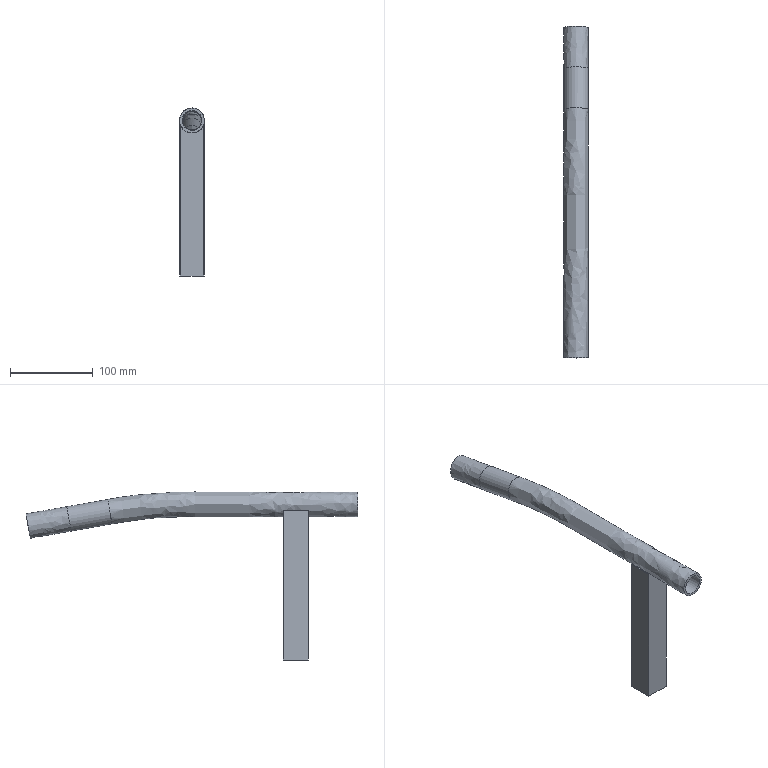Part | NX | features solid 2 | 1 solid | 22 faces | box 30 x 400.326 x 202.586 mm | volume 133159 mm3 | plane 15 | spline 4 | cylinder 3 | commonest cylinder face diameters 30 x2 24 x1
STEP:
#1=CARTESIAN_POINT('',(-482.491,1164.,-350.));
#2=VERTEX_POINT('',#1);
#3=CARTESIAN_POINT('',(-456.509,1164.,-350.));
#4=VERTEX_POINT('',#3);
#5=CARTESIAN_POINT('',(-482.491,1164.,-350.));
#6=CARTESIAN_POINT('',(-481.169,1164.,-352.288));
#7=CARTESIAN_POINT('',(-477.363,1164.,-356.084));
#8=CARTESIAN_POINT('',(-469.496,1164.,-358.205));
#9=CARTESIAN_POINT('',(-461.661,1164.,-356.096));
#10=CARTESIAN_POINT('',(-457.831,1164.,-352.288));
#11=CARTESIAN_POINT('',(-456.509,1164.,-350.));
#12=B_SPLINE_CURVE_WITH_KNOTS('',3,(#5,#6,#7,#8,#9,#10,#11),.UNSPECIFIED.,.F.,.F.,(4,1,1,1,4),(0.,0.007815,0.01563,0.02344,0.03126),.UNSPECIFIED.);
#13=EDGE_CURVE('',#2,#4,#12,.T.);
#14=ORIENTED_EDGE('',*,*,#13,.T.);
#15=CARTESIAN_POINT('',(-454.5,1164.,-350.));
#16=VERTEX_POINT('',#15);
#17=CARTESIAN_POINT('',(-454.5,1164.,-350.));
#18=DIRECTION('',(1.,0.,0.));
#19=VECTOR('',#18,1000.);
#20=LINE('',#17,#19);
#21=EDGE_CURVE('',#16,#4,#20,.F.);
#22=ORIENTED_EDGE('',*,*,#21,.F.);
#23=CARTESIAN_POINT('',(-454.5,1164.,-530.));
#24=VERTEX_POINT('',#23);
#25=CARTESIAN_POINT('',(-454.5,1164.,-635.));
#26=DIRECTION('',(0.,0.,1.));
#27=VECTOR('',#26,1000.);
#28=LINE('',#25,#27);
#29=EDGE_CURVE('',#24,#16,#28,.T.);
#30=ORIENTED_EDGE('',*,*,#29,.F.);
#31=CARTESIAN_POINT('',(-484.5,1164.,-530.));
#32=VERTEX_POINT('',#31);
#33=CARTESIAN_POINT('',(-451.75,1164.,-530.));
#34=DIRECTION('',(1.,0.,0.));
#35=VECTOR('',#34,1000.);
#36=LINE('',#33,#35);
#37=EDGE_CURVE('',#24,#32,#36,.F.);
#38=ORIENTED_EDGE('',*,*,#37,.T.);
#39=CARTESIAN_POINT('',(-484.5,1164.,-350.));
#40=VERTEX_POINT('',#39);
#41=CARTESIAN_POINT('',(-484.5,1164.,-635.));
#42=DIRECTION('',(0.,0.,-1.));
#43=VECTOR('',#42,1000.);
#44=LINE('',#41,#43);
#45=EDGE_CURVE('',#32,#40,#44,.F.);
#46=ORIENTED_EDGE('',*,*,#45,.T.);
#47=CARTESIAN_POINT('',(-454.5,1164.,-350.));
#48=DIRECTION('',(1.,0.,0.));
#49=VECTOR('',#48,1000.);
#50=LINE('',#47,#49);
#51=EDGE_CURVE('',#2,#40,#50,.F.);
#52=ORIENTED_EDGE('',*,*,#51,.F.);
#53=EDGE_LOOP('',(#14,#22,#30,#38,#46,#52));
#54=FACE_BOUND('',#53,.T.);
#55=CARTESIAN_POINT('',(-451.75,1164.,-635.));
#56=DIRECTION('',(0.,-1.,0.));
#57=DIRECTION('',(-1.,0.,0.));
#58=AXIS2_PLACEMENT_3D('',#55,#56,#57);
#59=PLANE('',#58);
#60=ADVANCED_FACE('',(#54),#59,.F.);
#61=CARTESIAN_POINT('',(-456.51,1162.5,-350.));
#62=VERTEX_POINT('',#61);
#63=CARTESIAN_POINT('',(-482.49,1162.5,-350.));
#64=VERTEX_POINT('',#63);
#65=CARTESIAN_POINT('',(-456.51,1162.5,-350.));
#66=CARTESIAN_POINT('',(-457.831,1162.5,-352.288));
#67=CARTESIAN_POINT('',(-461.637,1162.5,-356.084));
#68=CARTESIAN_POINT('',(-469.504,1162.5,-358.205));
#69=CARTESIAN_POINT('',(-477.339,1162.5,-356.096));
#70=CARTESIAN_POINT('',(-481.169,1162.5,-352.288));
#71=CARTESIAN_POINT('',(-482.49,1162.5,-350.));
#72=B_SPLINE_CURVE_WITH_KNOTS('',3,(#65,#66,#67,#68,#69,#70,#71),.UNSPECIFIED.,.F.,.F.,(4,1,1,1,4),(0.,0.007814,0.01563,0.02344,0.03126),.UNSPECIFIED.);
#73=EDGE_CURVE('',#62,#64,#72,.T.);
#74=ORIENTED_EDGE('',*,*,#73,.T.);
#75=CARTESIAN_POINT('',(-483.,1162.5,-350.));
#76=VERTEX_POINT('',#75);
#77=CARTESIAN_POINT('',(-451.75,1162.5,-350.));
#78=DIRECTION('',(1.,0.,0.));
#79=VECTOR('',#78,1000.);
#80=LINE('',#77,#79);
#81=EDGE_CURVE('',#76,#64,#80,.T.);
#82=ORIENTED_EDGE('',*,*,#81,.F.);
#83=CARTESIAN_POINT('',(-483.,1162.5,-530.));
#84=VERTEX_POINT('',#83);
#85=CARTESIAN_POINT('',(-483.,1162.5,-285.));
#86=DIRECTION('',(0.,0.,-1.));
#87=VECTOR('',#86,1000.);
#88=LINE('',#85,#87);
#89=EDGE_CURVE('',#76,#84,#88,.T.);
#90=ORIENTED_EDGE('',*,*,#89,.T.);
#91=CARTESIAN_POINT('',(-456.,1162.5,-530.));
#92=VERTEX_POINT('',#91);
#93=CARTESIAN_POINT('',(-451.75,1162.5,-530.));
#94=DIRECTION('',(-1.,0.,0.));
#95=VECTOR('',#94,1000.);
#96=LINE('',#93,#95);
#97=EDGE_CURVE('',#84,#92,#96,.F.);
#98=ORIENTED_EDGE('',*,*,#97,.T.);
#99=CARTESIAN_POINT('',(-456.,1162.5,-350.));
#100=VERTEX_POINT('',#99);
#101=CARTESIAN_POINT('',(-456.,1162.5,-285.));
#102=DIRECTION('',(0.,0.,-1.));
#103=VECTOR('',#102,1000.);
#104=LINE('',#101,#103);
#105=EDGE_CURVE('',#100,#92,#104,.T.);
#106=ORIENTED_EDGE('',*,*,#105,.F.);
#107=CARTESIAN_POINT('',(-451.75,1162.5,-350.));
#108=DIRECTION('',(1.,0.,0.));
#109=VECTOR('',#108,1000.);
#110=LINE('',#107,#109);
#111=EDGE_CURVE('',#62,#100,#110,.T.);
#112=ORIENTED_EDGE('',*,*,#111,.F.);
#113=EDGE_LOOP('',(#74,#82,#90,#98,#106,#112));
#114=FACE_BOUND('',#113,.T.);
#115=CARTESIAN_POINT('',(-451.75,1162.5,-285.));
#116=DIRECTION('',(0.,1.,0.));
#117=DIRECTION('',(1.,0.,0.));
#118=AXIS2_PLACEMENT_3D('',#115,#116,#117);
#119=PLANE('',#118);
#120=ADVANCED_FACE('',(#114),#119,.F.);
#121=CARTESIAN_POINT('',(-482.491,1164.,-350.));
#122=CARTESIAN_POINT('',(-482.49,1163.5,-350.));
#123=CARTESIAN_POINT('',(-482.49,1163.,-350.));
#124=CARTESIAN_POINT('',(-482.49,1162.5,-350.));
#125=B_SPLINE_CURVE_WITH_KNOTS('',3,(#121,#122,#123,#124),.UNSPECIFIED.,.F.,.F.,(4,4),(0.,0.0015),.UNSPECIFIED.);
#126=EDGE_CURVE('',#64,#2,#125,.F.);
#127=ORIENTED_EDGE('',*,*,#126,.T.);
#128=ORIENTED_EDGE('',*,*,#51,.T.);
#129=CARTESIAN_POINT('',(-484.5,1134.,-350.));
#130=VERTEX_POINT('',#129);
#131=CARTESIAN_POINT('',(-484.5,1134.,-350.));
#132=DIRECTION('',(0.,1.,0.));
#133=VECTOR('',#132,1000.);
#134=LINE('',#131,#133);
#135=EDGE_CURVE('',#40,#130,#134,.F.);
#136=ORIENTED_EDGE('',*,*,#135,.T.);
#137=CARTESIAN_POINT('',(-482.49,1134.,-350.));
#138=VERTEX_POINT('',#137);
#139=CARTESIAN_POINT('',(-454.5,1134.,-350.));
#140=DIRECTION('',(1.,0.,0.));
#141=VECTOR('',#140,1000.);
#142=LINE('',#139,#141);
#143=EDGE_CURVE('',#138,#130,#142,.F.);
#144=ORIENTED_EDGE('',*,*,#143,.F.);
#145=CARTESIAN_POINT('',(-482.49,1135.5,-350.));
#146=VERTEX_POINT('',#145);
#147=CARTESIAN_POINT('',(-482.49,764.,-350.));
#148=DIRECTION('',(0.,1.,0.));
#149=VECTOR('',#148,1000.);
#150=LINE('',#147,#149);
#151=EDGE_CURVE('',#138,#146,#150,.T.);
#152=ORIENTED_EDGE('',*,*,#151,.T.);
#153=CARTESIAN_POINT('',(-483.,1135.5,-350.));
#154=VERTEX_POINT('',#153);
#155=CARTESIAN_POINT('',(-451.75,1135.5,-350.));
#156=DIRECTION('',(1.,0.,0.));
#157=VECTOR('',#156,1000.);
#158=LINE('',#155,#157);
#159=EDGE_CURVE('',#154,#146,#158,.T.);
#160=ORIENTED_EDGE('',*,*,#159,.F.);
#161=CARTESIAN_POINT('',(-483.,1134.,-350.));
#162=DIRECTION('',(0.,-1.,0.));
#163=VECTOR('',#162,1000.);
#164=LINE('',#161,#163);
#165=EDGE_CURVE('',#76,#154,#164,.T.);
#166=ORIENTED_EDGE('',*,*,#165,.F.);
#167=ORIENTED_EDGE('',*,*,#81,.T.);
#168=EDGE_LOOP('',(#127,#128,#136,#144,#152,#160,#166,#167));
#169=FACE_BOUND('',#168,.T.);
#170=CARTESIAN_POINT('',(-454.5,1134.,-350.));
#171=DIRECTION('',(0.,0.,-1.));
#172=DIRECTION('',(0.,-1.,0.));
#173=AXIS2_PLACEMENT_3D('',#170,#171,#172);
#174=PLANE('',#173);
#175=ADVANCED_FACE('',(#169),#174,.F.);
#176=CARTESIAN_POINT('',(-456.509,1164.,-350.));
#177=CARTESIAN_POINT('',(-456.51,1163.5,-350.));
#178=CARTESIAN_POINT('',(-456.51,1163.,-350.));
#179=CARTESIAN_POINT('',(-456.51,1162.5,-350.));
#180=B_SPLINE_CURVE_WITH_KNOTS('',3,(#176,#177,#178,#179),.UNSPECIFIED.,.F.,.F.,(4,4),(0.,0.0015),.UNSPECIFIED.);
#181=EDGE_CURVE('',#4,#62,#180,.T.);
#182=ORIENTED_EDGE('',*,*,#181,.T.);
#183=ORIENTED_EDGE('',*,*,#111,.T.);
#184=CARTESIAN_POINT('',(-456.,1135.5,-350.));
#185=VERTEX_POINT('',#184);
#186=CARTESIAN_POINT('',(-456.,1134.,-350.));
#187=DIRECTION('',(0.,-1.,0.));
#188=VECTOR('',#187,1000.);
#189=LINE('',#186,#188);
#190=EDGE_CURVE('',#100,#185,#189,.T.);
#191=ORIENTED_EDGE('',*,*,#190,.T.);
#192=CARTESIAN_POINT('',(-456.51,1135.5,-350.));
#193=VERTEX_POINT('',#192);
#194=CARTESIAN_POINT('',(-451.75,1135.5,-350.));
#195=DIRECTION('',(1.,0.,0.));
#196=VECTOR('',#195,1000.);
#197=LINE('',#194,#196);
#198=EDGE_CURVE('',#193,#185,#197,.T.);
#199=ORIENTED_EDGE('',*,*,#198,.F.);
#200=CARTESIAN_POINT('',(-456.51,1134.,-350.));
#201=VERTEX_POINT('',#200);
#202=CARTESIAN_POINT('',(-456.51,764.,-350.));
#203=DIRECTION('',(0.,1.,0.));
#204=VECTOR('',#203,1000.);
#205=LINE('',#202,#204);
#206=EDGE_CURVE('',#193,#201,#205,.F.);
#207=ORIENTED_EDGE('',*,*,#206,.T.);
#208=CARTESIAN_POINT('',(-454.5,1134.,-350.));
#209=VERTEX_POINT('',#208);
#210=CARTESIAN_POINT('',(-454.5,1134.,-350.));
#211=DIRECTION('',(1.,0.,0.));
#212=VECTOR('',#211,1000.);
#213=LINE('',#210,#212);
#214=EDGE_CURVE('',#209,#201,#213,.F.);
#215=ORIENTED_EDGE('',*,*,#214,.F.);
#216=CARTESIAN_POINT('',(-454.5,1134.,-350.));
#217=DIRECTION('',(0.,-1.,0.));
#218=VECTOR('',#217,1000.);
#219=LINE('',#216,#218);
#220=EDGE_CURVE('',#209,#16,#219,.F.);
#221=ORIENTED_EDGE('',*,*,#220,.T.);
#222=ORIENTED_EDGE('',*,*,#21,.T.);
#223=EDGE_LOOP('',(#182,#183,#191,#199,#207,#215,#221,#222));
#224=FACE_BOUND('',#223,.T.);
#225=CARTESIAN_POINT('',(-454.5,1134.,-350.));
#226=DIRECTION('',(0.,0.,-1.));
#227=DIRECTION('',(0.,-1.,0.));
#228=AXIS2_PLACEMENT_3D('',#225,#226,#227);
#229=PLANE('',#228);
#230=ADVANCED_FACE('',(#224),#229,.F.);
#231=CARTESIAN_POINT('',(-454.5,1134.,-530.));
#232=VERTEX_POINT('',#231);
#233=CARTESIAN_POINT('',(-454.5,1134.,-530.));
#234=DIRECTION('',(0.,-1.,0.));
#235=VECTOR('',#234,1000.);
#236=LINE('',#233,#235);
#237=EDGE_CURVE('',#232,#24,#236,.F.);
#238=ORIENTED_EDGE('',*,*,#237,.F.);
#239=CARTESIAN_POINT('',(-484.5,1134.,-530.));
#240=VERTEX_POINT('',#239);
#241=CARTESIAN_POINT('',(-451.75,1134.,-530.));
#242=DIRECTION('',(1.,0.,0.));
#243=VECTOR('',#242,1000.);
#244=LINE('',#241,#243);
#245=EDGE_CURVE('',#232,#240,#244,.F.);
#246=ORIENTED_EDGE('',*,*,#245,.T.);
#247=CARTESIAN_POINT('',(-484.5,1134.,-530.));
#248=DIRECTION('',(0.,1.,0.));
#249=VECTOR('',#248,1000.);
#250=LINE('',#247,#249);
#251=EDGE_CURVE('',#240,#32,#250,.T.);
#252=ORIENTED_EDGE('',*,*,#251,.T.);
#253=ORIENTED_EDGE('',*,*,#37,.F.);
#254=EDGE_LOOP('',(#238,#246,#252,#253));
#255=FACE_BOUND('',#254,.T.);
#256=CARTESIAN_POINT('',(-483.,1135.5,-530.));
#257=VERTEX_POINT('',#256);
#258=CARTESIAN_POINT('',(-483.,1134.,-530.));
#259=DIRECTION('',(0.,1.,0.));
#260=VECTOR('',#259,1000.);
#261=LINE('',#258,#260);
#262=EDGE_CURVE('',#84,#257,#261,.F.);
#263=ORIENTED_EDGE('',*,*,#262,.T.);
#264=CARTESIAN_POINT('',(-456.,1135.5,-530.));
#265=VERTEX_POINT('',#264);
#266=CARTESIAN_POINT('',(-451.75,1135.5,-530.));
#267=DIRECTION('',(-1.,0.,0.));
#268=VECTOR('',#267,1000.);
#269=LINE('',#266,#268);
#270=EDGE_CURVE('',#257,#265,#269,.F.);
#271=ORIENTED_EDGE('',*,*,#270,.T.);
#272=CARTESIAN_POINT('',(-456.,1134.,-530.));
#273=DIRECTION('',(0.,1.,0.));
#274=VECTOR('',#273,1000.);
#275=LINE('',#272,#274);
#276=EDGE_CURVE('',#92,#265,#275,.F.);
#277=ORIENTED_EDGE('',*,*,#276,.F.);
#278=ORIENTED_EDGE('',*,*,#97,.F.);
#279=EDGE_LOOP('',(#263,#271,#277,#278));
#280=FACE_BOUND('',#279,.T.);
#281=CARTESIAN_POINT('',(-451.75,1134.,-530.));
#282=DIRECTION('',(0.,0.,-1.));
#283=DIRECTION('',(-1.,0.,0.));
#284=AXIS2_PLACEMENT_3D('',#281,#282,#283);
#285=PLANE('',#284);
#286=ADVANCED_FACE('',(#255,#280),#285,.T.);
#287=ORIENTED_EDGE('',*,*,#45,.F.);
#288=ORIENTED_EDGE('',*,*,#251,.F.);
#289=CARTESIAN_POINT('',(-484.5,1134.,-635.));
#290=DIRECTION('',(0.,0.,-1.));
#291=VECTOR('',#290,1000.);
#292=LINE('',#289,#291);
#293=EDGE_CURVE('',#240,#130,#292,.F.);
#294=ORIENTED_EDGE('',*,*,#293,.T.);
#295=ORIENTED_EDGE('',*,*,#135,.F.);
#296=EDGE_LOOP('',(#287,#288,#294,#295));
#297=FACE_BOUND('',#296,.T.);
#298=CARTESIAN_POINT('',(-484.5,1134.,-635.));
#299=DIRECTION('',(-1.,0.,0.));
#300=DIRECTION('',(0.,0.,1.));
#301=AXIS2_PLACEMENT_3D('',#298,#299,#300);
#302=PLANE('',#301);
#303=ADVANCED_FACE('',(#297),#302,.T.);
#304=CARTESIAN_POINT('',(-454.5,1134.,-635.));
#305=DIRECTION('',(0.,0.,1.));
#306=VECTOR('',#305,1000.);
#307=LINE('',#304,#306);
#308=EDGE_CURVE('',#232,#209,#307,.T.);
#309=ORIENTED_EDGE('',*,*,#308,.F.);
#310=ORIENTED_EDGE('',*,*,#237,.T.);
#311=ORIENTED_EDGE('',*,*,#29,.T.);
#312=ORIENTED_EDGE('',*,*,#220,.F.);
#313=EDGE_LOOP('',(#309,#310,#311,#312));
#314=FACE_BOUND('',#313,.T.);
#315=CARTESIAN_POINT('',(-454.5,1134.,-635.));
#316=DIRECTION('',(-1.,0.,0.));
#317=DIRECTION('',(0.,0.,1.));
#318=AXIS2_PLACEMENT_3D('',#315,#316,#317);
#319=PLANE('',#318);
#320=ADVANCED_FACE('',(#314),#319,.F.);
#321=ORIENTED_EDGE('',*,*,#214,.T.);
#322=CARTESIAN_POINT('',(-469.5,1134.,-342.5));
#323=DIRECTION('',(0.,1.,0.));
#324=DIRECTION('',(-1.,0.,0.));
#325=AXIS2_PLACEMENT_3D('',#322,#323,#324);
#326=CIRCLE('',#325,15.);
#327=EDGE_CURVE('',#201,#138,#326,.T.);
#328=ORIENTED_EDGE('',*,*,#327,.T.);
#329=ORIENTED_EDGE('',*,*,#143,.T.);
#330=ORIENTED_EDGE('',*,*,#293,.F.);
#331=ORIENTED_EDGE('',*,*,#245,.F.);
#332=ORIENTED_EDGE('',*,*,#308,.T.);
#333=EDGE_LOOP('',(#321,#328,#329,#330,#331,#332));
#334=FACE_BOUND('',#333,.T.);
#335=CARTESIAN_POINT('',(-451.75,1134.,-635.));
#336=DIRECTION('',(0.,-1.,0.));
#337=DIRECTION('',(-1.,0.,0.));
#338=AXIS2_PLACEMENT_3D('',#335,#336,#337);
#339=PLANE('',#338);
#340=ADVANCED_FACE('',(#334),#339,.T.);
#341=ORIENTED_EDGE('',*,*,#165,.T.);
#342=CARTESIAN_POINT('',(-483.,1135.5,-285.));
#343=DIRECTION('',(0.,0.,-1.));
#344=VECTOR('',#343,1000.);
#345=LINE('',#342,#344);
#346=EDGE_CURVE('',#154,#257,#345,.T.);
#347=ORIENTED_EDGE('',*,*,#346,.T.);
#348=ORIENTED_EDGE('',*,*,#262,.F.);
#349=ORIENTED_EDGE('',*,*,#89,.F.);
#350=EDGE_LOOP('',(#341,#347,#348,#349));
#351=FACE_BOUND('',#350,.T.);
#352=CARTESIAN_POINT('',(-483.,1134.,-285.));
#353=DIRECTION('',(1.,0.,0.));
#354=DIRECTION('',(0.,-1.,0.));
#355=AXIS2_PLACEMENT_3D('',#352,#353,#354);
#356=PLANE('',#355);
#357=ADVANCED_FACE('',(#351),#356,.T.);
#358=ORIENTED_EDGE('',*,*,#105,.T.);
#359=ORIENTED_EDGE('',*,*,#276,.T.);
#360=CARTESIAN_POINT('',(-456.,1135.5,-285.));
#361=DIRECTION('',(0.,0.,-1.));
#362=VECTOR('',#361,1000.);
#363=LINE('',#360,#362);
#364=EDGE_CURVE('',#185,#265,#363,.T.);
#365=ORIENTED_EDGE('',*,*,#364,.F.);
#366=ORIENTED_EDGE('',*,*,#190,.F.);
#367=EDGE_LOOP('',(#358,#359,#365,#366));
#368=FACE_BOUND('',#367,.T.);
#369=CARTESIAN_POINT('',(-456.,1134.,-285.));
#370=DIRECTION('',(1.,0.,0.));
#371=DIRECTION('',(0.,-1.,0.));
#372=AXIS2_PLACEMENT_3D('',#369,#370,#371);
#373=PLANE('',#372);
#374=ADVANCED_FACE('',(#368),#373,.F.);
#375=ORIENTED_EDGE('',*,*,#159,.T.);
#376=CARTESIAN_POINT('',(-469.5,1135.5,-342.5));
#377=DIRECTION('',(0.,-1.,0.));
#378=DIRECTION('',(1.,0.,0.));
#379=AXIS2_PLACEMENT_3D('',#376,#377,#378);
#380=CIRCLE('',#379,15.);
#381=EDGE_CURVE('',#146,#193,#380,.T.);
#382=ORIENTED_EDGE('',*,*,#381,.T.);
#383=ORIENTED_EDGE('',*,*,#198,.T.);
#384=ORIENTED_EDGE('',*,*,#364,.T.);
#385=ORIENTED_EDGE('',*,*,#270,.F.);
#386=ORIENTED_EDGE('',*,*,#346,.F.);
#387=EDGE_LOOP('',(#375,#382,#383,#384,#385,#386));
#388=FACE_BOUND('',#387,.T.);
#389=CARTESIAN_POINT('',(-451.75,1135.5,-285.));
#390=DIRECTION('',(0.,1.,0.));
#391=DIRECTION('',(1.,0.,0.));
#392=AXIS2_PLACEMENT_3D('',#389,#390,#391);
#393=PLANE('',#392);
#394=ADVANCED_FACE('',(#388),#393,.T.);
#395=ORIENTED_EDGE('',*,*,#381,.F.);
#396=ORIENTED_EDGE('',*,*,#151,.F.);
#397=ORIENTED_EDGE('',*,*,#327,.F.);
#398=ORIENTED_EDGE('',*,*,#206,.F.);
#399=EDGE_LOOP('',(#395,#396,#397,#398));
#400=FACE_BOUND('',#399,.T.);
#401=CARTESIAN_POINT('',(-469.5,764.,-342.5));
#402=DIRECTION('',(0.,1.,0.));
#403=DIRECTION('',(1.,0.,0.));
#404=AXIS2_PLACEMENT_3D('',#401,#402,#403);
#405=CYLINDRICAL_SURFACE('',#404,15.);
#406=ADVANCED_FACE('',(#400),#405,.F.);
#407=CARTESIAN_POINT('',(-484.417,1074.,-344.075));
#408=VERTEX_POINT('',#407);
#409=CARTESIAN_POINT('',(-483.008,1074.,-349.869));
#410=CARTESIAN_POINT('',(-485.422,1074.,-342.193));
#411=CARTESIAN_POINT('',(-482.422,1074.,-332.049));
#412=CARTESIAN_POINT('',(-471.256,1074.,-325.971));
#413=CARTESIAN_POINT('',(-459.051,1074.,-329.569));
#414=CARTESIAN_POINT('',(-452.971,1074.,-340.753));
#415=CARTESIAN_POINT('',(-456.566,1074.,-352.937));
#416=CARTESIAN_POINT('',(-467.74,1074.,-359.035));
#417=CARTESIAN_POINT('',(-477.899,1074.,-356.018));
#418=CARTESIAN_POINT('',(-483.008,1074.,-349.869));
#419=CARTESIAN_POINT('',(-485.422,1074.,-342.193));
#420=CARTESIAN_POINT('',(-482.422,1074.,-332.049));
#421=B_SPLINE_CURVE_WITH_KNOTS('',3,(#409,#410,#411,#412,#413,#414,#415,#416,#417,#418,#419,#420),.UNSPECIFIED.,.T.,.F.,(1,1,1,1,1,1,1,1,1,1,1,1,1,1,1,1),(-0.02345,-0.01172,-0.005861,0.,0.01172,0.02345,0.03517,0.04689,0.05861,0.07034,0.08206,0.08792,0.09378,0.1055,0.1172,0.129),.UNSPECIFIED.);
#422=EDGE_CURVE('',#408,#408,#421,.T.);
#423=ORIENTED_EDGE('',*,*,#422,.T.);
#424=EDGE_LOOP('',(#423));
#425=FACE_BOUND('',#424,.T.);
#426=CARTESIAN_POINT('',(-454.5,1373.241,-351.177));
#427=VERTEX_POINT('',#426);
#428=CARTESIAN_POINT('',(-484.5,1373.241,-351.177));
#429=VERTEX_POINT('',#428);
#430=CARTESIAN_POINT('',(-454.5,1373.241,-351.177));
#431=CARTESIAN_POINT('',(-454.501,1372.897,-353.128));
#432=CARTESIAN_POINT('',(-455.286,1372.22,-356.97));
#433=CARTESIAN_POINT('',(-459.727,1371.06,-363.546));
#434=CARTESIAN_POINT('',(-469.485,1370.356,-367.54));
#435=CARTESIAN_POINT('',(-481.251,1371.2,-362.754));
#436=CARTESIAN_POINT('',(-484.499,1372.562,-355.032));
#437=CARTESIAN_POINT('',(-484.5,1373.241,-351.177));
#438=B_SPLINE_CURVE_WITH_KNOTS('',3,(#430,#431,#432,#433,#434,#435,#436,#437),.UNSPECIFIED.,.F.,.F.,(4,1,1,1,1,4),(0.000005601,0.005866,0.01173,0.02345,0.03517,0.04689),.UNSPECIFIED.);
#439=EDGE_CURVE('',#427,#429,#438,.T.);
#440=ORIENTED_EDGE('',*,*,#439,.F.);
#441=CARTESIAN_POINT('',(-484.5,1373.241,-351.177));
#442=CARTESIAN_POINT('',(-484.501,1373.921,-347.32));
#443=CARTESIAN_POINT('',(-481.266,1375.281,-339.61));
#444=CARTESIAN_POINT('',(-469.515,1376.13,-334.795));
#445=CARTESIAN_POINT('',(-457.752,1375.282,-339.605));
#446=CARTESIAN_POINT('',(-454.498,1373.93,-347.273));
#447=CARTESIAN_POINT('',(-454.5,1373.241,-351.177));
#448=B_SPLINE_CURVE_WITH_KNOTS('',3,(#441,#442,#443,#444,#445,#446,#447),.UNSPECIFIED.,.F.,.F.,(4,1,1,1,4),(0.04689,0.05862,0.07034,0.08206,0.09379),.UNSPECIFIED.);
#449=EDGE_CURVE('',#429,#427,#448,.T.);
#450=ORIENTED_EDGE('',*,*,#449,.F.);
#451=EDGE_LOOP('',(#440,#450));
#452=FACE_BOUND('',#451,.T.);
#453=ORIENTED_EDGE('',*,*,#73,.F.);
#454=ORIENTED_EDGE('',*,*,#181,.F.);
#455=ORIENTED_EDGE('',*,*,#13,.F.);
#456=ORIENTED_EDGE('',*,*,#126,.F.);
#457=EDGE_LOOP('',(#453,#454,#455,#456));
#458=FACE_BOUND('',#457,.T.);
#459=CARTESIAN_POINT('',(-454.5,1074.,-337.197));
#460=CARTESIAN_POINT('',(-454.5,1103.148,-337.197));
#461=CARTESIAN_POINT('',(-454.5,1146.87,-337.193));
#462=CARTESIAN_POINT('',(-454.5,1205.165,-337.202));
#463=CARTESIAN_POINT('',(-454.5,1241.586,-337.198));
#464=CARTESIAN_POINT('',(-454.5,1270.761,-337.064));
#465=CARTESIAN_POINT('',(-454.5,1300.089,-337.334));
#466=CARTESIAN_POINT('',(-454.5,1329.539,-339.218));
#467=CARTESIAN_POINT('',(-454.5,1357.275,-342.994));
#468=CARTESIAN_POINT('',(-454.5,1370.26,-345.257));
#469=CARTESIAN_POINT('',(-454.5,1376.026,-346.278));
#470=CARTESIAN_POINT('',(-454.5,1074.,-347.803));
#471=CARTESIAN_POINT('',(-454.5,1103.148,-347.803));
#472=CARTESIAN_POINT('',(-454.5,1146.869,-347.8));
#473=CARTESIAN_POINT('',(-454.5,1205.165,-347.809));
#474=CARTESIAN_POINT('',(-454.5,1241.611,-347.805));
#475=CARTESIAN_POINT('',(-454.5,1270.737,-347.671));
#476=CARTESIAN_POINT('',(-454.5,1299.701,-347.937));
#477=CARTESIAN_POINT('',(-454.5,1328.483,-349.779));
#478=CARTESIAN_POINT('',(-454.5,1355.656,-353.478));
#479=CARTESIAN_POINT('',(-454.5,1368.533,-355.723));
#480=CARTESIAN_POINT('',(-454.5,1374.267,-356.738));
#481=CARTESIAN_POINT('',(-457.152,1074.,-354.848));
#482=CARTESIAN_POINT('',(-457.152,1103.148,-354.848));
#483=CARTESIAN_POINT('',(-457.152,1146.869,-354.845));
#484=CARTESIAN_POINT('',(-457.152,1205.165,-354.854));
#485=CARTESIAN_POINT('',(-457.152,1241.628,-354.85));
#486=CARTESIAN_POINT('',(-457.152,1270.721,-354.716));
#487=CARTESIAN_POINT('',(-457.152,1299.443,-354.98));
#488=CARTESIAN_POINT('',(-457.152,1327.782,-356.794));
#489=CARTESIAN_POINT('',(-457.152,1354.581,-360.442));
#490=CARTESIAN_POINT('',(-457.152,1367.387,-362.674));
#491=CARTESIAN_POINT('',(-457.152,1373.098,-363.686));
#492=CARTESIAN_POINT('',(-464.197,1074.,-357.5));
#493=CARTESIAN_POINT('',(-464.197,1103.148,-357.5));
#494=CARTESIAN_POINT('',(-464.197,1146.869,-357.497));
#495=CARTESIAN_POINT('',(-464.197,1205.165,-357.506));
#496=CARTESIAN_POINT('',(-464.197,1241.634,-357.502));
#497=CARTESIAN_POINT('',(-464.197,1270.715,-357.368));
#498=CARTESIAN_POINT('',(-464.197,1299.346,-357.631));
#499=CARTESIAN_POINT('',(-464.197,1327.519,-359.434));
#500=CARTESIAN_POINT('',(-464.197,1354.177,-363.063));
#501=CARTESIAN_POINT('',(-464.197,1366.955,-365.291));
#502=CARTESIAN_POINT('',(-464.197,1372.658,-366.301));
#503=CARTESIAN_POINT('',(-474.803,1074.,-357.5));
#504=CARTESIAN_POINT('',(-474.803,1103.148,-357.5));
#505=CARTESIAN_POINT('',(-474.803,1146.869,-357.497));
#506=CARTESIAN_POINT('',(-474.803,1205.165,-357.506));
#507=CARTESIAN_POINT('',(-474.803,1241.634,-357.502));
#508=CARTESIAN_POINT('',(-474.803,1270.715,-357.368));
#509=CARTESIAN_POINT('',(-474.803,1299.346,-357.631));
#510=CARTESIAN_POINT('',(-474.803,1327.519,-359.434));
#511=CARTESIAN_POINT('',(-474.803,1354.177,-363.063));
#512=CARTESIAN_POINT('',(-474.803,1366.955,-365.291));
#513=CARTESIAN_POINT('',(-474.803,1372.658,-366.301));
#514=CARTESIAN_POINT('',(-481.848,1074.,-354.848));
#515=CARTESIAN_POINT('',(-481.848,1103.148,-354.848));
#516=CARTESIAN_POINT('',(-481.848,1146.869,-354.845));
#517=CARTESIAN_POINT('',(-481.848,1205.165,-354.854));
#518=CARTESIAN_POINT('',(-481.848,1241.628,-354.85));
#519=CARTESIAN_POINT('',(-481.848,1270.721,-354.716));
#520=CARTESIAN_POINT('',(-481.848,1299.443,-354.98));
#521=CARTESIAN_POINT('',(-481.848,1327.782,-356.794));
#522=CARTESIAN_POINT('',(-481.848,1354.581,-360.442));
#523=CARTESIAN_POINT('',(-481.848,1367.387,-362.674));
#524=CARTESIAN_POINT('',(-481.848,1373.098,-363.686));
#525=CARTESIAN_POINT('',(-484.5,1074.,-347.803));
#526=CARTESIAN_POINT('',(-484.5,1103.148,-347.803));
#527=CARTESIAN_POINT('',(-484.5,1146.869,-347.8));
#528=CARTESIAN_POINT('',(-484.5,1205.165,-347.809));
#529=CARTESIAN_POINT('',(-484.5,1241.611,-347.805));
#530=CARTESIAN_POINT('',(-484.5,1270.737,-347.671));
#531=CARTESIAN_POINT('',(-484.5,1299.701,-347.937));
#532=CARTESIAN_POINT('',(-484.5,1328.483,-349.779));
#533=CARTESIAN_POINT('',(-484.5,1355.656,-353.478));
#534=CARTESIAN_POINT('',(-484.5,1368.533,-355.723));
#535=CARTESIAN_POINT('',(-484.5,1374.267,-356.738));
#536=CARTESIAN_POINT('',(-484.5,1074.,-337.197));
#537=CARTESIAN_POINT('',(-484.5,1103.148,-337.197));
#538=CARTESIAN_POINT('',(-484.5,1146.87,-337.193));
#539=CARTESIAN_POINT('',(-484.5,1205.165,-337.202));
#540=CARTESIAN_POINT('',(-484.5,1241.586,-337.198));
#541=CARTESIAN_POINT('',(-484.5,1270.761,-337.064));
#542=CARTESIAN_POINT('',(-484.5,1300.089,-337.334));
#543=CARTESIAN_POINT('',(-484.5,1329.539,-339.218));
#544=CARTESIAN_POINT('',(-484.5,1357.275,-342.994));
#545=CARTESIAN_POINT('',(-484.5,1370.26,-345.257));
#546=CARTESIAN_POINT('',(-484.5,1376.026,-346.278));
#547=CARTESIAN_POINT('',(-481.848,1074.,-330.152));
#548=CARTESIAN_POINT('',(-481.848,1103.147,-330.152));
#549=CARTESIAN_POINT('',(-481.848,1146.87,-330.148));
#550=CARTESIAN_POINT('',(-481.848,1205.165,-330.157));
#551=CARTESIAN_POINT('',(-481.848,1241.57,-330.153));
#552=CARTESIAN_POINT('',(-481.848,1270.778,-330.019));
#553=CARTESIAN_POINT('',(-481.848,1300.346,-330.291));
#554=CARTESIAN_POINT('',(-481.848,1330.24,-332.204));
#555=CARTESIAN_POINT('',(-481.848,1358.35,-336.03));
#556=CARTESIAN_POINT('',(-481.848,1371.407,-338.305));
#557=CARTESIAN_POINT('',(-481.848,1377.194,-339.33));
#558=CARTESIAN_POINT('',(-474.803,1074.,-327.5));
#559=CARTESIAN_POINT('',(-474.803,1103.147,-327.5));
#560=CARTESIAN_POINT('',(-474.803,1146.87,-327.497));
#561=CARTESIAN_POINT('',(-474.803,1205.165,-327.506));
#562=CARTESIAN_POINT('',(-474.803,1241.564,-327.502));
#563=CARTESIAN_POINT('',(-474.803,1270.784,-327.368));
#564=CARTESIAN_POINT('',(-474.803,1300.443,-327.64));
#565=CARTESIAN_POINT('',(-474.803,1330.503,-329.564));
#566=CARTESIAN_POINT('',(-474.803,1358.755,-333.409));
#567=CARTESIAN_POINT('',(-474.803,1371.839,-335.689));
#568=CARTESIAN_POINT('',(-474.803,1377.634,-336.715));
#569=CARTESIAN_POINT('',(-464.197,1074.,-327.5));
#570=CARTESIAN_POINT('',(-464.197,1103.147,-327.5));
#571=CARTESIAN_POINT('',(-464.197,1146.87,-327.497));
#572=CARTESIAN_POINT('',(-464.197,1205.165,-327.506));
#573=CARTESIAN_POINT('',(-464.197,1241.564,-327.502));
#574=CARTESIAN_POINT('',(-464.197,1270.784,-327.368));
#575=CARTESIAN_POINT('',(-464.197,1300.443,-327.64));
#576=CARTESIAN_POINT('',(-464.197,1330.503,-329.564));
#577=CARTESIAN_POINT('',(-464.197,1358.755,-333.409));
#578=CARTESIAN_POINT('',(-464.197,1371.839,-335.689));
#579=CARTESIAN_POINT('',(-464.197,1377.634,-336.715));
#580=CARTESIAN_POINT('',(-457.152,1074.,-330.152));
#581=CARTESIAN_POINT('',(-457.152,1103.147,-330.152));
#582=CARTESIAN_POINT('',(-457.152,1146.87,-330.148));
#583=CARTESIAN_POINT('',(-457.152,1205.165,-330.157));
#584=CARTESIAN_POINT('',(-457.152,1241.57,-330.153));
#585=CARTESIAN_POINT('',(-457.152,1270.778,-330.019));
#586=CARTESIAN_POINT('',(-457.152,1300.346,-330.291));
#587=CARTESIAN_POINT('',(-457.152,1330.24,-332.204));
#588=CARTESIAN_POINT('',(-457.152,1358.35,-336.03));
#589=CARTESIAN_POINT('',(-457.152,1371.407,-338.305));
#590=CARTESIAN_POINT('',(-457.152,1377.194,-339.33));
#591=CARTESIAN_POINT('',(-454.5,1074.,-337.197));
#592=CARTESIAN_POINT('',(-454.5,1103.148,-337.197));
#593=CARTESIAN_POINT('',(-454.5,1146.87,-337.193));
#594=CARTESIAN_POINT('',(-454.5,1205.165,-337.202));
#595=CARTESIAN_POINT('',(-454.5,1241.586,-337.198));
#596=CARTESIAN_POINT('',(-454.5,1270.761,-337.064));
#597=CARTESIAN_POINT('',(-454.5,1300.089,-337.334));
#598=CARTESIAN_POINT('',(-454.5,1329.539,-339.218));
#599=CARTESIAN_POINT('',(-454.5,1357.275,-342.994));
#600=CARTESIAN_POINT('',(-454.5,1370.26,-345.257));
#601=CARTESIAN_POINT('',(-454.5,1376.026,-346.278));
#602=CARTESIAN_POINT('',(-454.5,1074.,-347.803));
#603=CARTESIAN_POINT('',(-454.5,1103.148,-347.803));
#604=CARTESIAN_POINT('',(-454.5,1146.869,-347.8));
#605=CARTESIAN_POINT('',(-454.5,1205.165,-347.809));
#606=CARTESIAN_POINT('',(-454.5,1241.611,-347.805));
#607=CARTESIAN_POINT('',(-454.5,1270.737,-347.671));
#608=CARTESIAN_POINT('',(-454.5,1299.701,-347.937));
#609=CARTESIAN_POINT('',(-454.5,1328.483,-349.779));
#610=CARTESIAN_POINT('',(-454.5,1355.656,-353.478));
#611=CARTESIAN_POINT('',(-454.5,1368.533,-355.723));
#612=CARTESIAN_POINT('',(-454.5,1374.267,-356.738));
#613=(BOUNDED_SURFACE()B_SPLINE_SURFACE(4,3,((#459,#460,#461,#462,#463,#464,#465,#466,#467,#468,#469),(#470,#471,#472,#473,#474,#475,#476,#477,#478,#479,#480),(#481,#482,#483,#484,#485,#486,#487,#488,#489,#490,#491),(#492,#493,#494,#495,#496,#497,#498,#499,#500,#501,#502),(#503,#504,#505,#506,#507,#508,#509,#510,#511,#512,#513),(#514,#515,#516,#517,#518,#519,#520,#521,#522,#523,#524),(#525,#526,#527,#528,#529,#530,#531,#532,#533,#534,#535),(#536,#537,#538,#539,#540,#541,#542,#543,#544,#545,#546),(#547,#548,#549,#550,#551,#552,#553,#554,#555,#556,#557),(#558,#559,#560,#561,#562,#563,#564,#565,#566,#567,#568),(#569,#570,#571,#572,#573,#574,#575,#576,#577,#578,#579),(#580,#581,#582,#583,#584,#585,#586,#587,#588,#589,#590),(#591,#592,#593,#594,#595,#596,#597,#598,#599,#600,#601),(#602,#603,#604,#605,#606,#607,#608,#609,#610,#611,#612)),.UNSPECIFIED.,.T.,.F.,.F.)B_SPLINE_SURFACE_WITH_KNOTS((2,3,3,3,3,3,2),(4,1,1,1,1,1,1,1,4),(-0.25,0.,0.25,0.5,0.75,1.,1.25),(0.,0.25,0.375,0.5,0.5625,0.625,0.75,0.8125,0.8626),.UNSPECIFIED.)GEOMETRIC_REPRESENTATION_ITEM()RATIONAL_B_SPLINE_SURFACE(((0.5858,0.5858,0.5858,0.5858,0.5858,0.5858,0.5858,0.5858,0.5858,0.5858,0.5858),(0.5858,0.5858,0.5858,0.5858,0.5858,0.5858,0.5858,0.5858,0.5858,0.5858,0.5858),(0.5523,0.5523,0.5523,0.5523,0.5523,0.5523,0.5523,0.5523,0.5523,0.5523,0.5523),(0.5858,0.5858,0.5858,0.5858,0.5858,0.5858,0.5858,0.5858,0.5858,0.5858,0.5858),(0.5858,0.5858,0.5858,0.5858,0.5858,0.5858,0.5858,0.5858,0.5858,0.5858,0.5858),(0.5523,0.5523,0.5523,0.5523,0.5523,0.5523,0.5523,0.5523,0.5523,0.5523,0.5523),(0.5858,0.5858,0.5858,0.5858,0.5858,0.5858,0.5858,0.5858,0.5858,0.5858,0.5858),(0.5858,0.5858,0.5858,0.5858,0.5858,0.5858,0.5858,0.5858,0.5858,0.5858,0.5858),(0.5523,0.5523,0.5523,0.5523,0.5523,0.5523,0.5523,0.5523,0.5523,0.5523,0.5523),(0.5858,0.5858,0.5858,0.5858,0.5858,0.5858,0.5858,0.5858,0.5858,0.5858,0.5858),(0.5858,0.5858,0.5858,0.5858,0.5858,0.5858,0.5858,0.5858,0.5858,0.5858,0.5858),(0.5523,0.5523,0.5523,0.5523,0.5523,0.5523,0.5523,0.5523,0.5523,0.5523,0.5523),(0.5858,0.5858,0.5858,0.5858,0.5858,0.5858,0.5858,0.5858,0.5858,0.5858,0.5858),(0.5858,0.5858,0.5858,0.5858,0.5858,0.5858,0.5858,0.5858,0.5858,0.5858,0.5858)))REPRESENTATION_ITEM('')SURFACE());
#614=ADVANCED_FACE('',(#425,#452,#458),#613,.T.);
#615=CARTESIAN_POINT('',(-469.5,1373.24,-351.182));
#616=DIRECTION('',(0.,-0.9848,0.1736));
#617=DIRECTION('',(0.,-0.1736,-0.9848));
#618=AXIS2_PLACEMENT_3D('',#615,#616,#617);
#619=CIRCLE('',#618,15.);
#620=EDGE_CURVE('',#427,#429,#619,.T.);
#621=ORIENTED_EDGE('',*,*,#620,.T.);
#622=ORIENTED_EDGE('',*,*,#449,.T.);
#623=EDGE_LOOP('',(#621,#622));
#624=FACE_BOUND('',#623,.T.);
#625=CARTESIAN_POINT('',(-469.5,1373.24,-351.182));
#626=DIRECTION('',(0.,-0.9848,0.1736));
#627=DIRECTION('',(0.,0.1736,0.9848));
#628=AXIS2_PLACEMENT_3D('',#625,#626,#627);
#629=PLANE('',#628);
#630=ADVANCED_FACE('',(#624),#629,.F.);
#631=CARTESIAN_POINT('',(-457.5,1373.242,-351.174));
#632=VERTEX_POINT('',#631);
#633=CARTESIAN_POINT('',(-460.103,1374.874,-341.915));
#634=CARTESIAN_POINT('',(-456.202,1373.242,-351.173));
#635=CARTESIAN_POINT('',(-460.09,1371.609,-360.436));
#636=CARTESIAN_POINT('',(-469.491,1370.931,-364.279));
#637=CARTESIAN_POINT('',(-478.897,1371.606,-360.449));
#638=CARTESIAN_POINT('',(-482.798,1373.239,-351.192));
#639=CARTESIAN_POINT('',(-478.91,1374.872,-341.929));
#640=CARTESIAN_POINT('',(-469.509,1375.55,-338.086));
#641=CARTESIAN_POINT('',(-460.103,1374.874,-341.915));
#642=CARTESIAN_POINT('',(-456.202,1373.242,-351.173));
#643=CARTESIAN_POINT('',(-460.09,1371.609,-360.436));
#644=B_SPLINE_CURVE_WITH_KNOTS('',3,(#633,#634,#635,#636,#637,#638,#639,#640,#641,#642,#643),.UNSPECIFIED.,.T.,.F.,(1,1,1,1,1,1,1,1,1,1,1,1,1,1,1),(0.3749,0.4999,0.6249,0.7499,0.8749,0.9999,1.125,1.25,1.375,1.5,1.625,1.75,1.875,2.,2.125),.UNSPECIFIED.);
#645=EDGE_CURVE('',#632,#632,#644,.T.);
#646=ORIENTED_EDGE('',*,*,#645,.T.);
#647=EDGE_LOOP('',(#646));
#648=FACE_BOUND('',#647,.T.);
#649=CARTESIAN_POINT('',(-481.434,1074.,-343.76));
#650=VERTEX_POINT('',#649);
#651=CARTESIAN_POINT('',(-477.856,1074.,-352.848));
#652=CARTESIAN_POINT('',(-482.728,1074.,-343.894));
#653=CARTESIAN_POINT('',(-479.834,1074.,-334.134));
#654=CARTESIAN_POINT('',(-470.906,1074.,-329.278));
#655=CARTESIAN_POINT('',(-461.14,1074.,-332.155));
#656=CARTESIAN_POINT('',(-456.277,1074.,-341.102));
#657=CARTESIAN_POINT('',(-459.154,1074.,-350.851));
#658=CARTESIAN_POINT('',(-468.09,1074.,-355.724));
#659=CARTESIAN_POINT('',(-477.856,1074.,-352.848));
#660=CARTESIAN_POINT('',(-482.728,1074.,-343.894));
#661=CARTESIAN_POINT('',(-479.834,1074.,-334.134));
#662=B_SPLINE_CURVE_WITH_KNOTS('',3,(#651,#652,#653,#654,#655,#656,#657,#658,#659,#660,#661),.UNSPECIFIED.,.T.,.F.,(1,1,1,1,1,1,1,1,1,1,1,1,1,1,1),(-0.02813,-0.01876,-0.009378,0.,0.009378,0.01876,0.02813,0.03751,0.04689,0.05627,0.06565,0.07503,0.0844,0.09378,0.1032),.UNSPECIFIED.);
#663=EDGE_CURVE('',#650,#650,#662,.T.);
#664=ORIENTED_EDGE('',*,*,#663,.F.);
#665=EDGE_LOOP('',(#664));
#666=FACE_BOUND('',#665,.T.);
#667=CARTESIAN_POINT('',(-457.5,1074.,-338.257));
#668=CARTESIAN_POINT('',(-457.5,1103.148,-338.257));
#669=CARTESIAN_POINT('',(-457.5,1146.87,-338.254));
#670=CARTESIAN_POINT('',(-457.5,1205.165,-338.263));
#671=CARTESIAN_POINT('',(-457.5,1241.589,-338.259));
#672=CARTESIAN_POINT('',(-457.5,1270.759,-338.125));
#673=CARTESIAN_POINT('',(-457.5,1300.05,-338.394));
#674=CARTESIAN_POINT('',(-457.5,1329.433,-340.274));
#675=CARTESIAN_POINT('',(-457.5,1357.104,-344.041));
#676=CARTESIAN_POINT('',(-457.5,1370.07,-346.3));
#677=CARTESIAN_POINT('',(-457.5,1375.824,-347.319));
#678=CARTESIAN_POINT('',(-457.5,1074.,-346.743));
#679=CARTESIAN_POINT('',(-457.5,1103.148,-346.743));
#680=CARTESIAN_POINT('',(-457.5,1146.869,-346.739));
#681=CARTESIAN_POINT('',(-457.5,1205.165,-346.748));
#682=CARTESIAN_POINT('',(-457.5,1241.609,-346.744));
#683=CARTESIAN_POINT('',(-457.5,1270.74,-346.611));
#684=CARTESIAN_POINT('',(-457.5,1299.74,-346.877));
#685=CARTESIAN_POINT('',(-457.5,1328.589,-348.723));
#686=CARTESIAN_POINT('',(-457.5,1355.81,-352.428));
#687=CARTESIAN_POINT('',(-457.5,1368.689,-354.673));
#688=CARTESIAN_POINT('',(-457.5,1374.416,-355.687));
#689=CARTESIAN_POINT('',(-459.621,1074.,-352.379));
#690=CARTESIAN_POINT('',(-459.621,1103.148,-352.379));
#691=CARTESIAN_POINT('',(-459.621,1146.869,-352.375));
#692=CARTESIAN_POINT('',(-459.621,1205.165,-352.384));
#693=CARTESIAN_POINT('',(-459.621,1241.622,-352.38));
#694=CARTESIAN_POINT('',(-459.621,1270.727,-352.247));
#695=CARTESIAN_POINT('',(-459.621,1299.534,-352.511));
#696=CARTESIAN_POINT('',(-459.621,1328.028,-354.335));
#697=CARTESIAN_POINT('',(-459.621,1354.95,-357.999));
#698=CARTESIAN_POINT('',(-459.621,1367.771,-360.234));
#699=CARTESIAN_POINT('',(-459.621,1373.482,-361.245));
#700=CARTESIAN_POINT('',(-465.257,1074.,-354.5));
#701=CARTESIAN_POINT('',(-465.257,1103.148,-354.5));
#702=CARTESIAN_POINT('',(-465.257,1146.869,-354.497));
#703=CARTESIAN_POINT('',(-465.257,1205.165,-354.506));
#704=CARTESIAN_POINT('',(-465.257,1241.627,-354.502));
#705=CARTESIAN_POINT('',(-465.257,1270.722,-354.368));
#706=CARTESIAN_POINT('',(-465.257,1299.456,-354.632));
#707=CARTESIAN_POINT('',(-465.257,1327.817,-356.447));
#708=CARTESIAN_POINT('',(-465.257,1354.626,-360.096));
#709=CARTESIAN_POINT('',(-465.257,1367.426,-362.327));
#710=CARTESIAN_POINT('',(-465.257,1373.13,-363.337));
#711=CARTESIAN_POINT('',(-473.743,1074.,-354.5));
#712=CARTESIAN_POINT('',(-473.743,1103.148,-354.5));
#713=CARTESIAN_POINT('',(-473.743,1146.869,-354.497));
#714=CARTESIAN_POINT('',(-473.743,1205.165,-354.506));
#715=CARTESIAN_POINT('',(-473.743,1241.627,-354.502));
#716=CARTESIAN_POINT('',(-473.743,1270.722,-354.368));
#717=CARTESIAN_POINT('',(-473.743,1299.456,-354.632));
#718=CARTESIAN_POINT('',(-473.743,1327.817,-356.447));
#719=CARTESIAN_POINT('',(-473.743,1354.626,-360.096));
#720=CARTESIAN_POINT('',(-473.743,1367.426,-362.327));
#721=CARTESIAN_POINT('',(-473.743,1373.13,-363.337));
#722=CARTESIAN_POINT('',(-479.379,1074.,-352.379));
#723=CARTESIAN_POINT('',(-479.379,1103.148,-352.379));
#724=CARTESIAN_POINT('',(-479.379,1146.869,-352.375));
#725=CARTESIAN_POINT('',(-479.379,1205.165,-352.384));
#726=CARTESIAN_POINT('',(-479.379,1241.622,-352.38));
#727=CARTESIAN_POINT('',(-479.379,1270.727,-352.247));
#728=CARTESIAN_POINT('',(-479.379,1299.534,-352.511));
#729=CARTESIAN_POINT('',(-479.379,1328.028,-354.335));
#730=CARTESIAN_POINT('',(-479.379,1354.95,-357.999));
#731=CARTESIAN_POINT('',(-479.379,1367.771,-360.234));
#732=CARTESIAN_POINT('',(-479.379,1373.482,-361.245));
#733=CARTESIAN_POINT('',(-481.5,1074.,-346.743));
#734=CARTESIAN_POINT('',(-481.5,1103.148,-346.743));
#735=CARTESIAN_POINT('',(-481.5,1146.869,-346.739));
#736=CARTESIAN_POINT('',(-481.5,1205.165,-346.748));
#737=CARTESIAN_POINT('',(-481.5,1241.609,-346.744));
#738=CARTESIAN_POINT('',(-481.5,1270.74,-346.611));
#739=CARTESIAN_POINT('',(-481.5,1299.74,-346.877));
#740=CARTESIAN_POINT('',(-481.5,1328.589,-348.723));
#741=CARTESIAN_POINT('',(-481.5,1355.81,-352.428));
#742=CARTESIAN_POINT('',(-481.5,1368.689,-354.673));
#743=CARTESIAN_POINT('',(-481.5,1374.416,-355.687));
#744=CARTESIAN_POINT('',(-481.5,1074.,-338.257));
#745=CARTESIAN_POINT('',(-481.5,1103.148,-338.257));
#746=CARTESIAN_POINT('',(-481.5,1146.87,-338.254));
#747=CARTESIAN_POINT('',(-481.5,1205.165,-338.263));
#748=CARTESIAN_POINT('',(-481.5,1241.589,-338.259));
#749=CARTESIAN_POINT('',(-481.5,1270.759,-338.125));
#750=CARTESIAN_POINT('',(-481.5,1300.05,-338.394));
#751=CARTESIAN_POINT('',(-481.5,1329.433,-340.274));
#752=CARTESIAN_POINT('',(-481.5,1357.104,-344.041));
#753=CARTESIAN_POINT('',(-481.5,1370.07,-346.3));
#754=CARTESIAN_POINT('',(-481.5,1375.824,-347.319));
#755=CARTESIAN_POINT('',(-479.379,1074.,-332.621));
#756=CARTESIAN_POINT('',(-479.379,1103.147,-332.621));
#757=CARTESIAN_POINT('',(-479.379,1146.87,-332.618));
#758=CARTESIAN_POINT('',(-479.379,1205.165,-332.627));
#759=CARTESIAN_POINT('',(-479.379,1241.576,-332.623));
#760=CARTESIAN_POINT('',(-479.379,1270.772,-332.489));
#761=CARTESIAN_POINT('',(-479.379,1300.256,-332.76));
#762=CARTESIAN_POINT('',(-479.379,1329.994,-334.663));
#763=CARTESIAN_POINT('',(-479.379,1357.964,-338.47));
#764=CARTESIAN_POINT('',(-479.379,1370.987,-340.739));
#765=CARTESIAN_POINT('',(-479.379,1376.758,-341.761));
#766=CARTESIAN_POINT('',(-473.743,1074.,-330.5));
#767=CARTESIAN_POINT('',(-473.743,1103.147,-330.5));
#768=CARTESIAN_POINT('',(-473.743,1146.87,-330.497));
#769=CARTESIAN_POINT('',(-473.743,1205.165,-330.506));
#770=CARTESIAN_POINT('',(-473.743,1241.571,-330.502));
#771=CARTESIAN_POINT('',(-473.743,1270.777,-330.368));
#772=CARTESIAN_POINT('',(-473.743,1300.333,-330.639));
#773=CARTESIAN_POINT('',(-473.743,1330.205,-332.551));
#774=CARTESIAN_POINT('',(-473.743,1358.288,-336.373));
#775=CARTESIAN_POINT('',(-473.743,1371.332,-338.646));
#776=CARTESIAN_POINT('',(-473.743,1377.11,-339.669));
#777=CARTESIAN_POINT('',(-465.257,1074.,-330.5));
#778=CARTESIAN_POINT('',(-465.257,1103.147,-330.5));
#779=CARTESIAN_POINT('',(-465.257,1146.87,-330.497));
#780=CARTESIAN_POINT('',(-465.257,1205.165,-330.506));
#781=CARTESIAN_POINT('',(-465.257,1241.571,-330.502));
#782=CARTESIAN_POINT('',(-465.257,1270.777,-330.368));
#783=CARTESIAN_POINT('',(-465.257,1300.333,-330.639));
#784=CARTESIAN_POINT('',(-465.257,1330.205,-332.551));
#785=CARTESIAN_POINT('',(-465.257,1358.288,-336.373));
#786=CARTESIAN_POINT('',(-465.257,1371.332,-338.646));
#787=CARTESIAN_POINT('',(-465.257,1377.11,-339.669));
#788=CARTESIAN_POINT('',(-459.621,1074.,-332.621));
#789=CARTESIAN_POINT('',(-459.621,1103.147,-332.621));
#790=CARTESIAN_POINT('',(-459.621,1146.87,-332.618));
#791=CARTESIAN_POINT('',(-459.621,1205.165,-332.627));
#792=CARTESIAN_POINT('',(-459.621,1241.576,-332.623));
#793=CARTESIAN_POINT('',(-459.621,1270.772,-332.489));
#794=CARTESIAN_POINT('',(-459.621,1300.256,-332.76));
#795=CARTESIAN_POINT('',(-459.621,1329.994,-334.663));
#796=CARTESIAN_POINT('',(-459.621,1357.964,-338.47));
#797=CARTESIAN_POINT('',(-459.621,1370.987,-340.739));
#798=CARTESIAN_POINT('',(-459.621,1376.758,-341.761));
#799=CARTESIAN_POINT('',(-457.5,1074.,-338.257));
#800=CARTESIAN_POINT('',(-457.5,1103.148,-338.257));
#801=CARTESIAN_POINT('',(-457.5,1146.87,-338.254));
#802=CARTESIAN_POINT('',(-457.5,1205.165,-338.263));
#803=CARTESIAN_POINT('',(-457.5,1241.589,-338.259));
#804=CARTESIAN_POINT('',(-457.5,1270.759,-338.125));
#805=CARTESIAN_POINT('',(-457.5,1300.05,-338.394));
#806=CARTESIAN_POINT('',(-457.5,1329.433,-340.274));
#807=CARTESIAN_POINT('',(-457.5,1357.104,-344.041));
#808=CARTESIAN_POINT('',(-457.5,1370.07,-346.3));
#809=CARTESIAN_POINT('',(-457.5,1375.824,-347.319));
#810=CARTESIAN_POINT('',(-457.5,1074.,-346.743));
#811=CARTESIAN_POINT('',(-457.5,1103.148,-346.743));
#812=CARTESIAN_POINT('',(-457.5,1146.869,-346.739));
#813=CARTESIAN_POINT('',(-457.5,1205.165,-346.748));
#814=CARTESIAN_POINT('',(-457.5,1241.609,-346.744));
#815=CARTESIAN_POINT('',(-457.5,1270.74,-346.611));
#816=CARTESIAN_POINT('',(-457.5,1299.74,-346.877));
#817=CARTESIAN_POINT('',(-457.5,1328.589,-348.723));
#818=CARTESIAN_POINT('',(-457.5,1355.81,-352.428));
#819=CARTESIAN_POINT('',(-457.5,1368.689,-354.673));
#820=CARTESIAN_POINT('',(-457.5,1374.416,-355.687));
#821=(BOUNDED_SURFACE()B_SPLINE_SURFACE(4,3,((#667,#668,#669,#670,#671,#672,#673,#674,#675,#676,#677),(#678,#679,#680,#681,#682,#683,#684,#685,#686,#687,#688),(#689,#690,#691,#692,#693,#694,#695,#696,#697,#698,#699),(#700,#701,#702,#703,#704,#705,#706,#707,#708,#709,#710),(#711,#712,#713,#714,#715,#716,#717,#718,#719,#720,#721),(#722,#723,#724,#725,#726,#727,#728,#729,#730,#731,#732),(#733,#734,#735,#736,#737,#738,#739,#740,#741,#742,#743),(#744,#745,#746,#747,#748,#749,#750,#751,#752,#753,#754),(#755,#756,#757,#758,#759,#760,#761,#762,#763,#764,#765),(#766,#767,#768,#769,#770,#771,#772,#773,#774,#775,#776),(#777,#778,#779,#780,#781,#782,#783,#784,#785,#786,#787),(#788,#789,#790,#791,#792,#793,#794,#795,#796,#797,#798),(#799,#800,#801,#802,#803,#804,#805,#806,#807,#808,#809),(#810,#811,#812,#813,#814,#815,#816,#817,#818,#819,#820)),.UNSPECIFIED.,.T.,.F.,.F.)B_SPLINE_SURFACE_WITH_KNOTS((2,3,3,3,3,3,2),(4,1,1,1,1,1,1,1,4),(-0.25,0.,0.25,0.5,0.75,1.,1.25),(0.,0.25,0.375,0.5,0.5625,0.625,0.75,0.8125,0.8625),.UNSPECIFIED.)GEOMETRIC_REPRESENTATION_ITEM()RATIONAL_B_SPLINE_SURFACE(((0.5858,0.5858,0.5858,0.5858,0.5858,0.5858,0.5858,0.5858,0.5858,0.5858,0.5858),(0.5858,0.5858,0.5858,0.5858,0.5858,0.5858,0.5858,0.5858,0.5858,0.5858,0.5858),(0.5523,0.5523,0.5523,0.5523,0.5523,0.5523,0.5523,0.5523,0.5523,0.5523,0.5523),(0.5858,0.5858,0.5858,0.5858,0.5858,0.5858,0.5858,0.5858,0.5858,0.5858,0.5858),(0.5858,0.5858,0.5858,0.5858,0.5858,0.5858,0.5858,0.5858,0.5858,0.5858,0.5858),(0.5523,0.5523,0.5523,0.5523,0.5523,0.5523,0.5523,0.5523,0.5523,0.5523,0.5523),(0.5858,0.5858,0.5858,0.5858,0.5858,0.5858,0.5858,0.5858,0.5858,0.5858,0.5858),(0.5858,0.5858,0.5858,0.5858,0.5858,0.5858,0.5858,0.5858,0.5858,0.5858,0.5858),(0.5523,0.5523,0.5523,0.5523,0.5523,0.5523,0.5523,0.5523,0.5523,0.5523,0.5523),(0.5858,0.5858,0.5858,0.5858,0.5858,0.5858,0.5858,0.5858,0.5858,0.5858,0.5858),(0.5858,0.5858,0.5858,0.5858,0.5858,0.5858,0.5858,0.5858,0.5858,0.5858,0.5858),(0.5523,0.5523,0.5523,0.5523,0.5523,0.5523,0.5523,0.5523,0.5523,0.5523,0.5523),(0.5858,0.5858,0.5858,0.5858,0.5858,0.5858,0.5858,0.5858,0.5858,0.5858,0.5858),(0.5858,0.5858,0.5858,0.5858,0.5858,0.5858,0.5858,0.5858,0.5858,0.5858,0.5858)))REPRESENTATION_ITEM('')SURFACE());
#822=ADVANCED_FACE('',(#648,#666),#821,.F.);
#823=CARTESIAN_POINT('',(-469.5,1373.24,-351.182));
#824=DIRECTION('',(0.,-0.9848,0.1736));
#825=DIRECTION('',(0.,-0.1736,-0.9848));
#826=AXIS2_PLACEMENT_3D('',#823,#824,#825);
#827=CIRCLE('',#826,15.);
#828=EDGE_CURVE('',#429,#427,#827,.T.);
#829=ORIENTED_EDGE('',*,*,#828,.T.);
#830=ORIENTED_EDGE('',*,*,#439,.T.);
#831=EDGE_LOOP('',(#829,#830));
#832=FACE_BOUND('',#831,.T.);
#833=CARTESIAN_POINT('',(-469.5,1373.24,-351.182));
#834=DIRECTION('',(0.,0.9848,-0.1736));
#835=DIRECTION('',(1.,0.,0.));
#836=AXIS2_PLACEMENT_3D('',#833,#834,#835);
#837=PLANE('',#836);
#838=ADVANCED_FACE('',(#832),#837,.F.);
#839=CARTESIAN_POINT('',(-481.5,1422.481,-359.865));
#840=VERTEX_POINT('',#839);
#841=CARTESIAN_POINT('',(-469.5,1422.481,-359.865));
#842=DIRECTION('',(0.,0.9848,-0.1736));
#843=DIRECTION('',(-1.,0.,0.));
#844=AXIS2_PLACEMENT_3D('',#841,#842,#843);
#845=CIRCLE('',#844,12.);
#846=EDGE_CURVE('',#840,#840,#845,.T.);
#847=ORIENTED_EDGE('',*,*,#846,.T.);
#848=EDGE_LOOP('',(#847));
#849=FACE_BOUND('',#848,.T.);
#850=ORIENTED_EDGE('',*,*,#645,.F.);
#851=EDGE_LOOP('',(#850));
#852=FACE_BOUND('',#851,.T.);
#853=CARTESIAN_POINT('',(-469.5,1422.481,-359.865));
#854=DIRECTION('',(0.,-0.9848,0.1736));
#855=DIRECTION('',(-1.,0.,0.));
#856=AXIS2_PLACEMENT_3D('',#853,#854,#855);
#857=CYLINDRICAL_SURFACE('',#856,12.);
#858=ADVANCED_FACE('',(#849,#852),#857,.F.);
#859=CARTESIAN_POINT('',(-454.5,1422.481,-359.865));
#860=VERTEX_POINT('',#859);
#861=CARTESIAN_POINT('',(-469.5,1422.481,-359.865));
#862=DIRECTION('',(0.,-0.9848,0.1736));
#863=DIRECTION('',(1.,0.,0.));
#864=AXIS2_PLACEMENT_3D('',#861,#862,#863);
#865=CIRCLE('',#864,15.);
#866=EDGE_CURVE('',#860,#860,#865,.T.);
#867=ORIENTED_EDGE('',*,*,#866,.T.);
#868=EDGE_LOOP('',(#867));
#869=FACE_BOUND('',#868,.T.);
#870=ORIENTED_EDGE('',*,*,#620,.F.);
#871=ORIENTED_EDGE('',*,*,#828,.F.);
#872=EDGE_LOOP('',(#870,#871));
#873=FACE_BOUND('',#872,.T.);
#874=CARTESIAN_POINT('',(-469.5,1422.481,-359.865));
#875=DIRECTION('',(0.,-0.9848,0.1736));
#876=DIRECTION('',(-1.,0.,0.));
#877=AXIS2_PLACEMENT_3D('',#874,#875,#876);
#878=CYLINDRICAL_SURFACE('',#877,15.);
#879=ADVANCED_FACE('',(#869,#873),#878,.T.);
#880=ORIENTED_EDGE('',*,*,#866,.F.);
#881=EDGE_LOOP('',(#880));
#882=FACE_BOUND('',#881,.T.);
#883=CARTESIAN_POINT('',(-469.5,1474.326,-353.775));
#884=VERTEX_POINT('',#883);
#885=CARTESIAN_POINT('',(-463.59,1474.188,-354.556));
#886=CARTESIAN_POINT('',(-471.478,1474.465,-352.986));
#887=CARTESIAN_POINT('',(-481.25,1473.762,-356.973));
#888=CARTESIAN_POINT('',(-486.122,1471.723,-368.536));
#889=CARTESIAN_POINT('',(-481.262,1469.681,-380.118));
#890=CARTESIAN_POINT('',(-469.502,1468.835,-384.916));
#891=CARTESIAN_POINT('',(-457.762,1469.678,-380.135));
#892=CARTESIAN_POINT('',(-452.871,1471.719,-368.561));
#893=CARTESIAN_POINT('',(-456.939,1473.418,-358.923));
#894=CARTESIAN_POINT('',(-463.59,1474.188,-354.556));
#895=CARTESIAN_POINT('',(-471.478,1474.465,-352.986));
#896=CARTESIAN_POINT('',(-481.25,1473.762,-356.973));
#897=B_SPLINE_CURVE_WITH_KNOTS('',3,(#885,#886,#887,#888,#889,#890,#891,#892,#893,#894,#895,#896),.UNSPECIFIED.,.T.,.F.,(1,1,1,1,1,1,1,1,1,1,1,1,1,1,1,1),(-0.02345,-0.01172,-0.005861,0.,0.01172,0.02345,0.03517,0.04689,0.05861,0.07034,0.08206,0.08792,0.09378,0.1055,0.1172,0.129),.UNSPECIFIED.);
#898=EDGE_CURVE('',#884,#884,#897,.T.);
#899=ORIENTED_EDGE('',*,*,#898,.T.);
#900=EDGE_LOOP('',(#899));
#901=FACE_BOUND('',#900,.T.);
#902=CARTESIAN_POINT('',(-454.5,1423.402,-354.642));
#903=CARTESIAN_POINT('',(-454.5,1439.922,-357.555));
#904=CARTESIAN_POINT('',(-454.5,1456.443,-360.468));
#905=CARTESIAN_POINT('',(-454.5,1472.964,-363.381));
#906=CARTESIAN_POINT('',(-454.5,1421.56,-365.088));
#907=CARTESIAN_POINT('',(-454.5,1438.076,-368.));
#908=CARTESIAN_POINT('',(-454.5,1454.592,-370.912));
#909=CARTESIAN_POINT('',(-454.5,1471.108,-373.824));
#910=CARTESIAN_POINT('',(-457.152,1420.337,-372.026));
#911=CARTESIAN_POINT('',(-457.152,1436.85,-374.937));
#912=CARTESIAN_POINT('',(-457.152,1453.363,-377.849));
#913=CARTESIAN_POINT('',(-457.152,1469.876,-380.761));
#914=CARTESIAN_POINT('',(-464.197,1419.876,-374.637));
#915=CARTESIAN_POINT('',(-464.197,1436.388,-377.548));
#916=CARTESIAN_POINT('',(-464.197,1452.9,-380.46));
#917=CARTESIAN_POINT('',(-464.197,1469.412,-383.371));
#918=CARTESIAN_POINT('',(-474.803,1419.876,-374.637));
#919=CARTESIAN_POINT('',(-474.803,1436.388,-377.548));
#920=CARTESIAN_POINT('',(-474.803,1452.9,-380.46));
#921=CARTESIAN_POINT('',(-474.803,1469.412,-383.371));
#922=CARTESIAN_POINT('',(-481.848,1420.337,-372.026));
#923=CARTESIAN_POINT('',(-481.848,1436.85,-374.937));
#924=CARTESIAN_POINT('',(-481.848,1453.363,-377.849));
#925=CARTESIAN_POINT('',(-481.848,1469.876,-380.761));
#926=CARTESIAN_POINT('',(-484.5,1421.56,-365.088));
#927=CARTESIAN_POINT('',(-484.5,1438.076,-368.));
#928=CARTESIAN_POINT('',(-484.5,1454.592,-370.912));
#929=CARTESIAN_POINT('',(-484.5,1471.108,-373.824));
#930=CARTESIAN_POINT('',(-484.5,1423.402,-354.642));
#931=CARTESIAN_POINT('',(-484.5,1439.922,-357.555));
#932=CARTESIAN_POINT('',(-484.5,1456.443,-360.468));
#933=CARTESIAN_POINT('',(-484.5,1472.964,-363.381));
#934=CARTESIAN_POINT('',(-481.848,1424.625,-347.704));
#935=CARTESIAN_POINT('',(-481.848,1441.149,-350.618));
#936=CARTESIAN_POINT('',(-481.848,1457.673,-353.531));
#937=CARTESIAN_POINT('',(-481.848,1474.197,-356.445));
#938=CARTESIAN_POINT('',(-474.803,1425.085,-345.093));
#939=CARTESIAN_POINT('',(-474.803,1441.61,-348.006));
#940=CARTESIAN_POINT('',(-474.803,1458.135,-350.92));
#941=CARTESIAN_POINT('',(-474.803,1474.66,-353.834));
#942=CARTESIAN_POINT('',(-464.197,1425.085,-345.093));
#943=CARTESIAN_POINT('',(-464.197,1441.61,-348.006));
#944=CARTESIAN_POINT('',(-464.197,1458.135,-350.92));
#945=CARTESIAN_POINT('',(-464.197,1474.66,-353.834));
#946=CARTESIAN_POINT('',(-457.152,1424.625,-347.704));
#947=CARTESIAN_POINT('',(-457.152,1441.149,-350.618));
#948=CARTESIAN_POINT('',(-457.152,1457.673,-353.531));
#949=CARTESIAN_POINT('',(-457.152,1474.197,-356.445));
#950=CARTESIAN_POINT('',(-454.5,1423.402,-354.642));
#951=CARTESIAN_POINT('',(-454.5,1439.922,-357.555));
#952=CARTESIAN_POINT('',(-454.5,1456.443,-360.468));
#953=CARTESIAN_POINT('',(-454.5,1472.964,-363.381));
#954=CARTESIAN_POINT('',(-454.5,1421.56,-365.088));
#955=CARTESIAN_POINT('',(-454.5,1438.076,-368.));
#956=CARTESIAN_POINT('',(-454.5,1454.592,-370.912));
#957=CARTESIAN_POINT('',(-454.5,1471.108,-373.824));
#958=(BOUNDED_SURFACE()B_SPLINE_SURFACE(4,3,((#902,#903,#904,#905),(#906,#907,#908,#909),(#910,#911,#912,#913),(#914,#915,#916,#917),(#918,#919,#920,#921),(#922,#923,#924,#925),(#926,#927,#928,#929),(#930,#931,#932,#933),(#934,#935,#936,#937),(#938,#939,#940,#941),(#942,#943,#944,#945),(#946,#947,#948,#949),(#950,#951,#952,#953),(#954,#955,#956,#957)),.UNSPECIFIED.,.T.,.F.,.F.)B_SPLINE_SURFACE_WITH_KNOTS((2,3,3,3,3,3,2),(4,4),(-0.25,0.,0.25,0.5,0.75,1.,1.25),(1.,1.144),.UNSPECIFIED.)GEOMETRIC_REPRESENTATION_ITEM()RATIONAL_B_SPLINE_SURFACE(((0.5858,0.5858,0.5858,0.5858),(0.5858,0.5858,0.5858,0.5858),(0.5523,0.5523,0.5523,0.5523),(0.5858,0.5858,0.5858,0.5858),(0.5858,0.5858,0.5858,0.5858),(0.5523,0.5523,0.5523,0.5523),(0.5858,0.5858,0.5858,0.5858),(0.5858,0.5858,0.5858,0.5858),(0.5523,0.5523,0.5523,0.5523),(0.5858,0.5858,0.5858,0.5858),(0.5858,0.5858,0.5858,0.5858),(0.5523,0.5523,0.5523,0.5523),(0.5858,0.5858,0.5858,0.5858),(0.5858,0.5858,0.5858,0.5858)))REPRESENTATION_ITEM('')SURFACE());
#959=ADVANCED_FACE('',(#882,#901),#958,.T.);
#960=ORIENTED_EDGE('',*,*,#898,.F.);
#961=EDGE_LOOP('',(#960));
#962=FACE_BOUND('',#961,.T.);
#963=CARTESIAN_POINT('',(-469.5,1473.805,-356.73));
#964=VERTEX_POINT('',#963);
#965=CARTESIAN_POINT('',(-460.086,1473.353,-359.294));
#966=CARTESIAN_POINT('',(-469.502,1474.031,-355.448));
#967=CARTESIAN_POINT('',(-478.904,1473.353,-359.291));
#968=CARTESIAN_POINT('',(-482.796,1471.723,-368.538));
#969=CARTESIAN_POINT('',(-478.91,1470.089,-377.804));
#970=CARTESIAN_POINT('',(-469.502,1469.412,-381.642));
#971=CARTESIAN_POINT('',(-460.109,1470.087,-377.817));
#972=CARTESIAN_POINT('',(-456.201,1471.719,-368.561));
#973=CARTESIAN_POINT('',(-460.086,1473.353,-359.294));
#974=CARTESIAN_POINT('',(-469.502,1474.031,-355.448));
#975=CARTESIAN_POINT('',(-478.904,1473.353,-359.291));
#976=B_SPLINE_CURVE_WITH_KNOTS('',3,(#965,#966,#967,#968,#969,#970,#971,#972,#973,#974,#975),.UNSPECIFIED.,.T.,.F.,(1,1,1,1,1,1,1,1,1,1,1,1,1,1,1),(-0.02813,-0.01876,-0.009378,0.,0.009378,0.01876,0.02813,0.03751,0.04689,0.05627,0.06565,0.07503,0.0844,0.09378,0.1032),.UNSPECIFIED.);
#977=EDGE_CURVE('',#964,#964,#976,.T.);
#978=ORIENTED_EDGE('',*,*,#977,.T.);
#979=EDGE_LOOP('',(#978));
#980=FACE_BOUND('',#979,.T.);
#981=CARTESIAN_POINT('',(-469.5,1471.721,-368.547));
#982=DIRECTION('',(0.,-0.9848,0.1736));
#983=DIRECTION('',(0.,0.1736,0.9848));
#984=AXIS2_PLACEMENT_3D('',#981,#982,#983);
#985=PLANE('',#984);
#986=ADVANCED_FACE('',(#962,#980),#985,.F.);
#987=ORIENTED_EDGE('',*,*,#846,.F.);
#988=EDGE_LOOP('',(#987));
#989=FACE_BOUND('',#988,.T.);
#990=ORIENTED_EDGE('',*,*,#977,.F.);
#991=EDGE_LOOP('',(#990));
#992=FACE_BOUND('',#991,.T.);
#993=CARTESIAN_POINT('',(-457.5,1423.218,-355.687));
#994=CARTESIAN_POINT('',(-457.5,1439.737,-358.599));
#995=CARTESIAN_POINT('',(-457.5,1456.256,-361.512));
#996=CARTESIAN_POINT('',(-457.5,1472.775,-364.425));
#997=CARTESIAN_POINT('',(-457.5,1421.744,-364.043));
#998=CARTESIAN_POINT('',(-457.5,1438.259,-366.955));
#999=CARTESIAN_POINT('',(-457.5,1454.775,-369.867));
#1000=CARTESIAN_POINT('',(-457.5,1471.29,-372.779));
#1001=CARTESIAN_POINT('',(-459.621,1420.765,-369.593));
#1002=CARTESIAN_POINT('',(-459.621,1437.278,-372.505));
#1003=CARTESIAN_POINT('',(-459.621,1453.791,-375.417));
#1004=CARTESIAN_POINT('',(-459.621,1470.304,-378.328));
#1005=CARTESIAN_POINT('',(-465.257,1420.397,-371.683));
#1006=CARTESIAN_POINT('',(-465.257,1436.909,-374.594));
#1007=CARTESIAN_POINT('',(-465.257,1453.421,-377.506));
#1008=CARTESIAN_POINT('',(-465.257,1469.933,-380.417));
#1009=CARTESIAN_POINT('',(-473.743,1420.397,-371.683));
#1010=CARTESIAN_POINT('',(-473.743,1436.909,-374.594));
#1011=CARTESIAN_POINT('',(-473.743,1453.421,-377.506));
#1012=CARTESIAN_POINT('',(-473.743,1469.933,-380.417));
#1013=CARTESIAN_POINT('',(-479.379,1420.765,-369.593));
#1014=CARTESIAN_POINT('',(-479.379,1437.278,-372.505));
#1015=CARTESIAN_POINT('',(-479.379,1453.791,-375.417));
#1016=CARTESIAN_POINT('',(-479.379,1470.304,-378.328));
#1017=CARTESIAN_POINT('',(-481.5,1421.744,-364.043));
#1018=CARTESIAN_POINT('',(-481.5,1438.259,-366.955));
#1019=CARTESIAN_POINT('',(-481.5,1454.775,-369.867));
#1020=CARTESIAN_POINT('',(-481.5,1471.29,-372.779));
#1021=CARTESIAN_POINT('',(-481.5,1423.218,-355.687));
#1022=CARTESIAN_POINT('',(-481.5,1439.737,-358.599));
#1023=CARTESIAN_POINT('',(-481.5,1456.256,-361.512));
#1024=CARTESIAN_POINT('',(-481.5,1472.775,-364.425));
#1025=CARTESIAN_POINT('',(-479.379,1424.196,-350.136));
#1026=CARTESIAN_POINT('',(-479.379,1440.718,-353.049));
#1027=CARTESIAN_POINT('',(-479.379,1457.239,-355.963));
#1028=CARTESIAN_POINT('',(-479.379,1473.761,-358.876));
#1029=CARTESIAN_POINT('',(-473.743,1424.565,-348.047));
#1030=CARTESIAN_POINT('',(-473.743,1441.087,-350.96));
#1031=CARTESIAN_POINT('',(-473.743,1457.609,-353.874));
#1032=CARTESIAN_POINT('',(-473.743,1474.132,-356.787));
#1033=CARTESIAN_POINT('',(-465.257,1424.565,-348.047));
#1034=CARTESIAN_POINT('',(-465.257,1441.087,-350.96));
#1035=CARTESIAN_POINT('',(-465.257,1457.609,-353.874));
#1036=CARTESIAN_POINT('',(-465.257,1474.132,-356.787));
#1037=CARTESIAN_POINT('',(-459.621,1424.196,-350.136));
#1038=CARTESIAN_POINT('',(-459.621,1440.718,-353.049));
#1039=CARTESIAN_POINT('',(-459.621,1457.239,-355.963));
#1040=CARTESIAN_POINT('',(-459.621,1473.761,-358.876));
#1041=CARTESIAN_POINT('',(-457.5,1423.218,-355.687));
#1042=CARTESIAN_POINT('',(-457.5,1439.737,-358.599));
#1043=CARTESIAN_POINT('',(-457.5,1456.256,-361.512));
#1044=CARTESIAN_POINT('',(-457.5,1472.775,-364.425));
#1045=CARTESIAN_POINT('',(-457.5,1421.744,-364.043));
#1046=CARTESIAN_POINT('',(-457.5,1438.259,-366.955));
#1047=CARTESIAN_POINT('',(-457.5,1454.775,-369.867));
#1048=CARTESIAN_POINT('',(-457.5,1471.29,-372.779));
#1049=(BOUNDED_SURFACE()B_SPLINE_SURFACE(4,3,((#993,#994,#995,#996),(#997,#998,#999,#1000),(#1001,#1002,#1003,#1004),(#1005,#1006,#1007,#1008),(#1009,#1010,#1011,#1012),(#1013,#1014,#1015,#1016),(#1017,#1018,#1019,#1020),(#1021,#1022,#1023,#1024),(#1025,#1026,#1027,#1028),(#1029,#1030,#1031,#1032),(#1033,#1034,#1035,#1036),(#1037,#1038,#1039,#1040),(#1041,#1042,#1043,#1044),(#1045,#1046,#1047,#1048)),.UNSPECIFIED.,.T.,.F.,.F.)B_SPLINE_SURFACE_WITH_KNOTS((2,3,3,3,3,3,2),(4,4),(-0.25,0.,0.25,0.5,0.75,1.,1.25),(1.,1.144),.UNSPECIFIED.)GEOMETRIC_REPRESENTATION_ITEM()RATIONAL_B_SPLINE_SURFACE(((0.5858,0.5858,0.5858,0.5858),(0.5858,0.5858,0.5858,0.5858),(0.5523,0.5523,0.5523,0.5523),(0.5858,0.5858,0.5858,0.5858),(0.5858,0.5858,0.5858,0.5858),(0.5523,0.5523,0.5523,0.5523),(0.5858,0.5858,0.5858,0.5858),(0.5858,0.5858,0.5858,0.5858),(0.5523,0.5523,0.5523,0.5523),(0.5858,0.5858,0.5858,0.5858),(0.5858,0.5858,0.5858,0.5858),(0.5523,0.5523,0.5523,0.5523),(0.5858,0.5858,0.5858,0.5858),(0.5858,0.5858,0.5858,0.5858)))REPRESENTATION_ITEM('')SURFACE());
#1050=ADVANCED_FACE('',(#989,#992),#1049,.F.);
#1051=ORIENTED_EDGE('',*,*,#422,.F.);
#1052=EDGE_LOOP('',(#1051));
#1053=FACE_BOUND('',#1052,.T.);
#1054=ORIENTED_EDGE('',*,*,#663,.T.);
#1055=EDGE_LOOP('',(#1054));
#1056=FACE_BOUND('',#1055,.T.);
#1057=CARTESIAN_POINT('',(-469.5,1074.,-342.5));
#1058=DIRECTION('',(0.,-1.,0.));
#1059=DIRECTION('',(-1.,0.,0.));
#1060=AXIS2_PLACEMENT_3D('',#1057,#1058,#1059);
#1061=PLANE('',#1060);
#1062=ADVANCED_FACE('',(#1053,#1056),#1061,.T.);
#1063=CLOSED_SHELL('',(#60,#120,#175,#230,#286,#303,#320,#340,#357,#374,#394,#406,#614,#630,#822,#838,#858,#879,#959,#986,#1050,#1062));
#1064=MANIFOLD_SOLID_BREP('',#1063);
#1065=(LENGTH_UNIT()NAMED_UNIT(*)SI_UNIT(.MILLI.,.METRE.));
#1066=UNCERTAINTY_MEASURE_WITH_UNIT(LENGTH_MEASURE(0.0508),#1065,'','');
#1067=(NAMED_UNIT(*)PLANE_ANGLE_UNIT()SI_UNIT($,.RADIAN.));
#1068=(NAMED_UNIT(*)SI_UNIT($,.STERADIAN.)SOLID_ANGLE_UNIT());
#1069=(GEOMETRIC_REPRESENTATION_CONTEXT(3)GLOBAL_UNCERTAINTY_ASSIGNED_CONTEXT((#1066))GLOBAL_UNIT_ASSIGNED_CONTEXT((#1065,#1067,#1068))REPRESENTATION_CONTEXT('',''));
#1070=ADVANCED_BREP_SHAPE_REPRESENTATION('',(#1064),#1069);